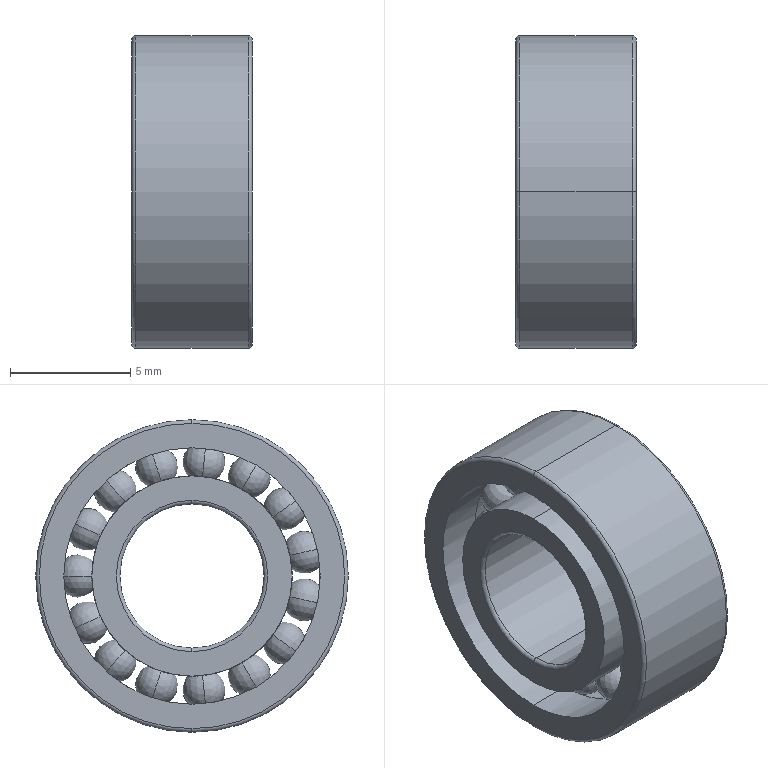Part | SolidWorks | features Stock 1 | 1 solid | 102 faces | box 5 x 13 x 13 mm | volume 374.773 mm3 | torus 56 | sphere 30 | cylinder 12 | plane 4 | commonest cylinder face diameters 8.333 x4 10.667 x4 6 x2 13 x2